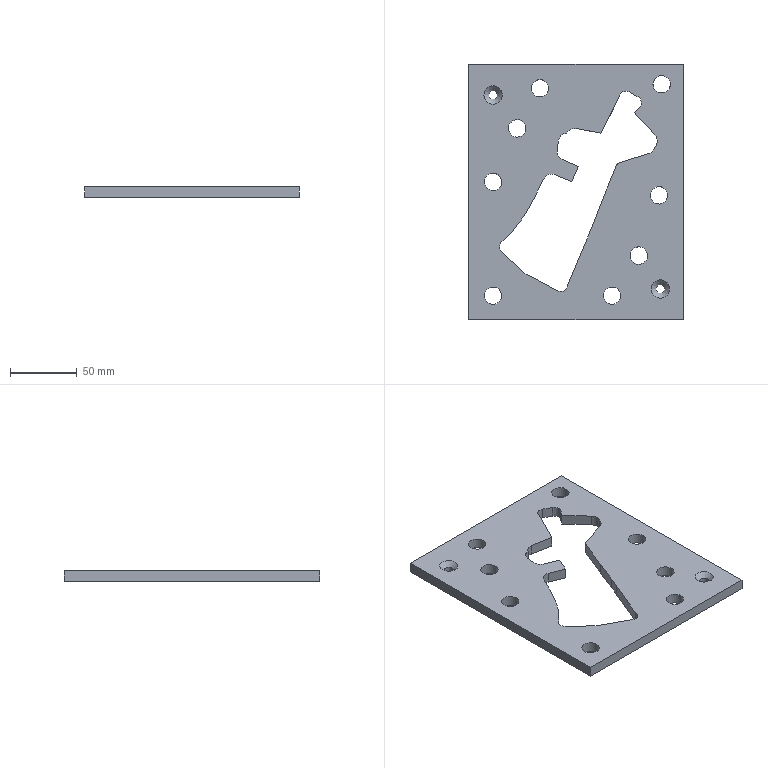Part | STEP file | gslz 2016.10.28-13_id750_x_t | 1 solid | 58 faces | box 160 x 191 x 8 mm | volume 181921 mm3 | plane 34 | cylinder 22 | cone 2 | commonest cylinder face diameters 13 x8 10 x5 6.5 x2 12 x2 14 x2 12.078 x1